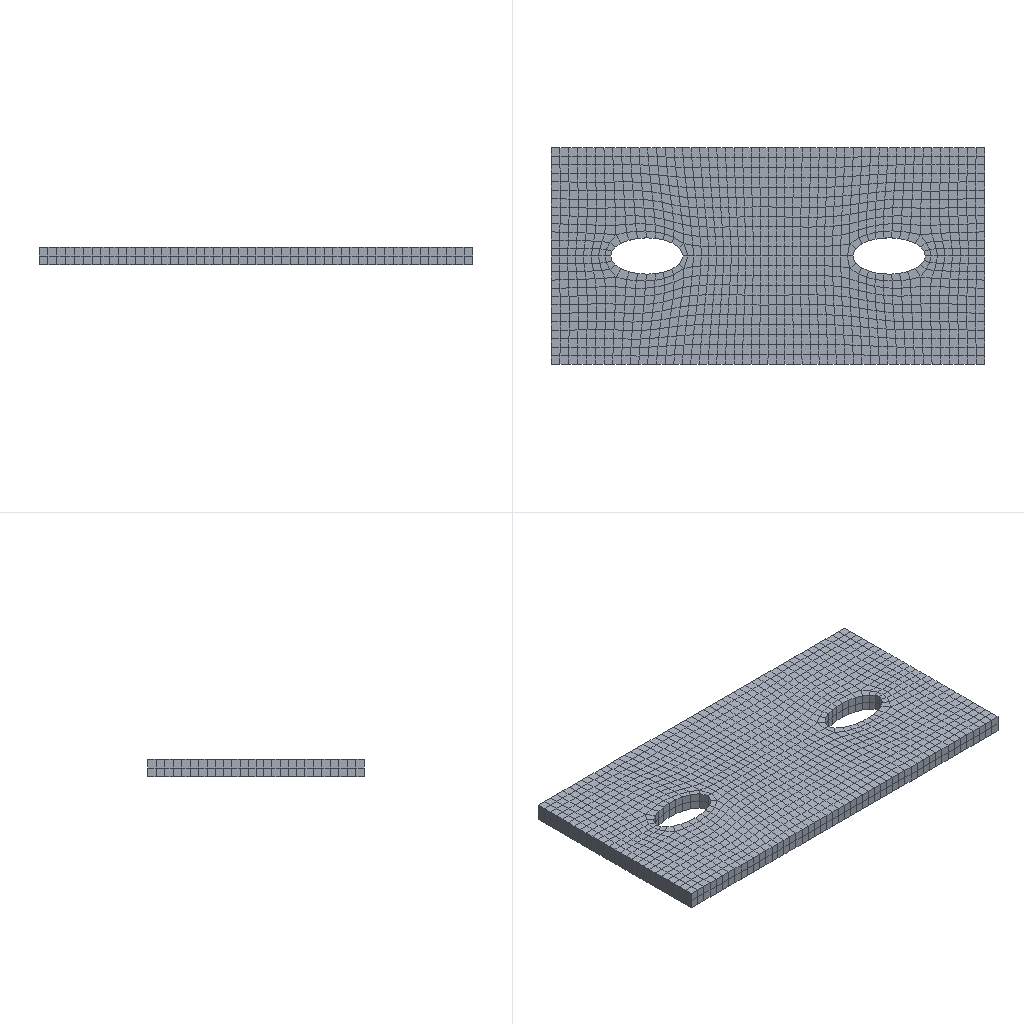Simulation study | abaqus
Set-up summary:
category,name,step,type,value,unit,region
solver,abaqus
solver,version,,,Abaqus/Standard 2020
units,not stated in the deck,,not stated
analysis,deck,,coupled temperature-displacement,coupled temperature-displacement
load_step,Step-1,Step-1,coupled temperature-displacement
load_step,requested,,,1
mesh,nodes,,,3810
mesh,elements,,,2344
element_type,Q3D8,,solid,2344
load,load commands in deck,,count,4
bc,support commands in deck,,count,4
material,MATERIAL-1,,in results
check,setup vs results,,match,"per instance, exact: element labels, types and connectivity; labels of the nodes the elements use; coordinates of those nodes at SINGLE_PRECISION in 1 of 1 instance(s)"
Abaqus input file, long lists of numbers shortened:
*Heading
** Job name: Job-1 Model name: Model-1
** Generated by: Abaqus/CAE 2020
*Preprint, echo=NO, model=NO, history=NO, contact=NO
**
** PARTS
**
*Part, name=work
*Node
      1,   43.135,        -12.5,           0.
      2,          50.,        -12.5,           0.
** (3808 more lines like these left out)
*Element, type=Q3D8
   1,  520,  529,   80,   79, 2816, 2825, 1596, 1597
   2,  529,  530,   81,   80, 2825, 2826, 1595, 1596
** (2342 more lines like these left out)
*Nset, nset=Set-3, generate
    1,  3810,     1
*Elset, elset=Set-3, generate
    1,  2344,     1
** Section: Section-1
*Solid Section, elset=Set-3, material=Material-1
,
*End Part
**
**
** ASSEMBLY
**
*Assembly, name=Assembly
**
*Instance, name=work-1, part=work
*End Instance
**
*Nset, nset=Set-1, instance=work-1
    3,    4,    5,    6,    9,   10,   13,   14,   17,   18,   19,   20,   73,   74,   75,   76
   77,   78,   79,   80,   81,   82,   83,   84,   85,   86,   87,   88,   89,   90,   91,   92
** (18 more lines like these left out)
*Elset, elset=Set-1, instance=work-1
    1,    2,    3,   67,   77,   87,   97,  107,  117,  127,  142,  152,  162,  172,  182,  183
  184,  185,  186,  187,  188,  189,  190,  191,  192,  294,  295,  296,  297,  359,  369,  379
** (11 more lines like these left out)
*Nset, nset=Set-6, instance=work-1
    3,    6,   13,   14,   73,   74,   75,   76,   77,   78,   79,   80,   81,   82,   83,   84
   85,   86,   87,   88,   89,   90,   91,   92,   93,   94,   95,   96,   97,   98,   99,  100
** (8 more lines like these left out)
*Elset, elset=Set-6, instance=work-1
    1,    2,    3,   67,   77,   87,   97,  107,  117,  127,  142,  152,  162,  172,  182,  183
  184,  185,  186,  187,  188,  189,  190,  191,  192,  294,  295,  296,  297,  359,  369,  379
** (5 more lines like these left out)
*Nset, nset=Set-9, instance=work-1
    4,    5,    9,   10,   21,   22,   23,   24,   25,   26,   27,   28,   29,   30,   31,   32
   33,   34,   35,   36,   37,   38,   39,   40,   41,   42,  154,  155,  159,  160,  161,  162
** (3 more lines like these left out)
*Elset, elset=Set-9, instance=work-1
  283,  284,  285,  286,  287,  288,  289,  290,  291,  292,  293,  338,  339,  340,  341,  342
  343,  344,  345,  346,  347,  348,  349,  869,  870,  871,  872,  873,  874,  875,  876,  877
** (4 more lines like these left out)
*Nset, nset=Set-10, instance=work-1
    2,    3,    6,    7,   12,   13,   14,   15,   17,   18,   19,   20,   61,   62,   63,   64
   65,   66,   67,   68,   69,   70,   71,   72,  122,  123,  124,  125,  126,  127,  128,  129
** (9 more lines like these left out)
*Elset, elset=Set-10, instance=work-1
   43,   50,   57,   58,   59,   60,   61,   62,   63,   64,   65,   66,   67,  499,  506,  513
  520,  527,  534,  541,  548,  555,  562,  563,  564,  565,  629,  636,  643,  644,  645,  646
** (5 more lines like these left out)
*Elset, elset=_Surf-1_S5, internal, instance=work-1
    1,    2,    3,  183,  184,  185,  186,  187,  188,  189,  190,  191,  192,  294,  295,  296
  297,  493,  494,  495,  496,  497,  498,  499,  587,  588,  589,  769,  770,  771,  772,  773
** (5 more lines like these left out)
*Elset, elset=_Surf-1_S4, internal, instance=work-1
   67,   77,   87,   97,  107,  117,  127,  142,  152,  162,  172,  182,  359,  369,  379,  389
  399,  409,  419,  429,  439,  449,  459,  472,  482,  492,  653,  663,  673,  683,  693,  703
** (5 more lines like these left out)
*Surface, type=ELEMENT, name=Surf-1
_Surf-1_S5, S5
_Surf-1_S4, S4
*Elset, elset=_Surf-2_S5, internal, instance=work-1
    1,    2,    3,  183,  184,  185,  186,  187,  188,  189,  190,  191,  192,  294,  295,  296
  297,  493,  494,  495,  496,  497,  498,  499,  587,  588,  589,  769,  770,  771,  772,  773
** (5 more lines like these left out)
*Elset, elset=_Surf-2_S4, internal, instance=work-1
   67,   77,   87,   97,  107,  117,  127,  142,  152,  162,  172,  182,  359,  369,  379,  389
  399,  409,  419,  429,  439,  449,  459,  472,  482,  492,  653,  663,  673,  683,  693,  703
** (5 more lines like these left out)
*Surface, type=ELEMENT, name=Surf-2
_Surf-2_S5, S5
_Surf-2_S4, S4
*Elset, elset=_Surf-3_S5, internal, instance=work-1
    1,    2,    3,  183,  184,  185,  186,  187,  188,  189,  190,  191,  192,  294,  295,  296
  297,  493,  494,  495,  496,  497,  498,  499,  587,  588,  589,  769,  770,  771,  772,  773
** (5 more lines like these left out)
*Elset, elset=_Surf-3_S4, internal, instance=work-1
   67,   77,   87,   97,  107,  117,  127,  142,  152,  162,  172,  182,  359,  369,  379,  389
  399,  409,  419,  429,  439,  449,  459,  472,  482,  492,  653,  663,  673,  683,  693,  703
** (5 more lines like these left out)
*Surface, type=ELEMENT, name=Surf-3
_Surf-3_S5, S5
_Surf-3_S4, S4
*Elset, elset=_Surf-4_S5, internal, instance=work-1
    1,    2,    3,  183,  184,  185,  186,  187,  188,  189,  190,  191,  192,  294,  295,  296
  297,  493,  494,  495,  496,  497,  498,  499,  587,  588,  589,  769,  770,  771,  772,  773
** (5 more lines like these left out)
*Elset, elset=_Surf-4_S4, internal, instance=work-1
   67,   77,   87,   97,  107,  117,  127,  142,  152,  162,  172,  182,  359,  369,  379,  389
  399,  409,  419,  429,  439,  449,  459,  472,  482,  492,  653,  663,  673,  683,  693,  703
** (5 more lines like these left out)
*Surface, type=ELEMENT, name=Surf-4
_Surf-4_S5, S5
_Surf-4_S4, S4
*Elset, elset=_Surf-5_S5, internal, instance=work-1
 1173, 1174, 1175, 1176, 1177, 1372, 1373, 1374, 1375, 1376, 1377, 1378, 1510, 1511, 1512, 1513
 1514, 1515, 1516, 1517, 1518, 1519, 1520, 1632, 1633, 1634, 1759, 1760, 1761, 1762, 1763, 1958
** (2 more lines like these left out)
*Elset, elset=_Surf-5_S4, internal, instance=work-1
 1248, 1258, 1268, 1278, 1288, 1298, 1308, 1318, 1328, 1338, 1351, 1361, 1371, 1479, 1489, 1499
 1509, 1698, 1708, 1718, 1728, 1738, 1748, 1758, 1834, 1844, 1854, 1864, 1874, 1884, 1894, 1904
** (1 more lines like these left out)
*Surface, type=ELEMENT, name=Surf-5
_Surf-5_S5, S5
_Surf-5_S4, S4
*Elset, elset=_Surf-6_S5, internal, instance=work-1
    1,    2,    3,  183,  184,  185,  186,  187,  188,  189,  190,  191,  192,  294,  295,  296
  297,  493,  494,  495,  496,  497,  498,  499,  587,  588,  589,  769,  770,  771,  772,  773
** (5 more lines like these left out)
*Elset, elset=_Surf-6_S4, internal, instance=work-1
   67,   77,   87,   97,  107,  117,  127,  142,  152,  162,  172,  182,  359,  369,  379,  389
  399,  409,  419,  429,  439,  449,  459,  472,  482,  492,  653,  663,  673,  683,  693,  703
** (5 more lines like these left out)
*Surface, type=ELEMENT, name=Surf-6
_Surf-6_S5, S5
_Surf-6_S4, S4
*End Assembly
*Amplitude, name=Amp-1, definition=PERIODIC
1,         188000.,              0.,              0.
             1.,              0.
*Amplitude, name=Amp-2
             0.,              0.,             10.,              1.
**
** MATERIALS
**
*Material, name=Material-1
*Conductivity
40.,
*Density
 1.67e-09,
*Elastic
70000., 0.33
*Electrical Conductivity
 0.02665,
*Expansion
 2.32e-06,
*Specific Heat
 8.9e+08,
**
** PHYSICAL CONSTANTS
**
*Physical Constants, absolute zero=-273., stefan boltzmann=5.67e-08
**
** BOUNDARY CONDITIONS
**
** Name: BC-4 Type: 对称/反对称/完全固定
*Boundary
Set-9, ENCASTRE
**
** PREDEFINED FIELDS
**
** Name: Predefined Field-1   Type: Temperature
*Initial Conditions, type=TEMPERATURE
Set-1, 20.
** ----------------------------------------------------------------
**
** STEP: Step-1
**
*Step, name=Step-1, nlgeom=YES, inc=1000
*Coupled Temperature-displacement, electrical, creep=none, deltmx=1e+20, stabilize=0.0002, allsdtol=0.05, continue=NO
0.1, 10., 0.0001, 10.
**
** BOUNDARY CONDITIONS
**
** Name: BC-3 Type: 电势
*Boundary
Set-9, 9, 9
**
** LOADS
**
** Name: Load-1   Type: Surface current
*Dsecurrent, amplitude=Amp-1
Surf-6,CS,1.
** Name: Load-2   Type: Pressure
*Dsload, amplitude=Amp-2
Surf-4, P, 0.1
**
** INTERACTIONS
**
** Interaction: Int-1
*Sfilm
Surf-1, F, 20., 0.01
** Interaction: Int-2
*Sradiate
Surf-2, R, 20., 0.5
**
** OUTPUT REQUESTS
**
*Restart, write, frequency=0
**
** FIELD OUTPUT: F-Output-1
**
*Output, field
*Node Output
CECHG, CECUR, EPOT, NT, RECUR, RF, RFL, RT
U
*Element Output, directions=YES
E, ECD, EPG, HFL, LE, MISES, MISESMAX, NCURS, PE, PEEQ, S, TEMP, VE, VEEQ
*Contact Output
ECD, ECDA, ECDT, ECDTA
**
** HISTORY OUTPUT: H-Output-1
**
*Output, history, variable=PRESELECT
*End Step
Results summary:
result,step,,completed,increments=12 time=10.0/10.0
result,analysis,,,"coupled temperature-displacement, steady state"
result,last_loadstep,,,1
result,primary field,,,"U, NT11"
result,reaction total,,FX,3.9e-05,model units
result,reaction total,,FY,-1.1e-05,model units
result,reaction total,,FZ,-0.0,model units